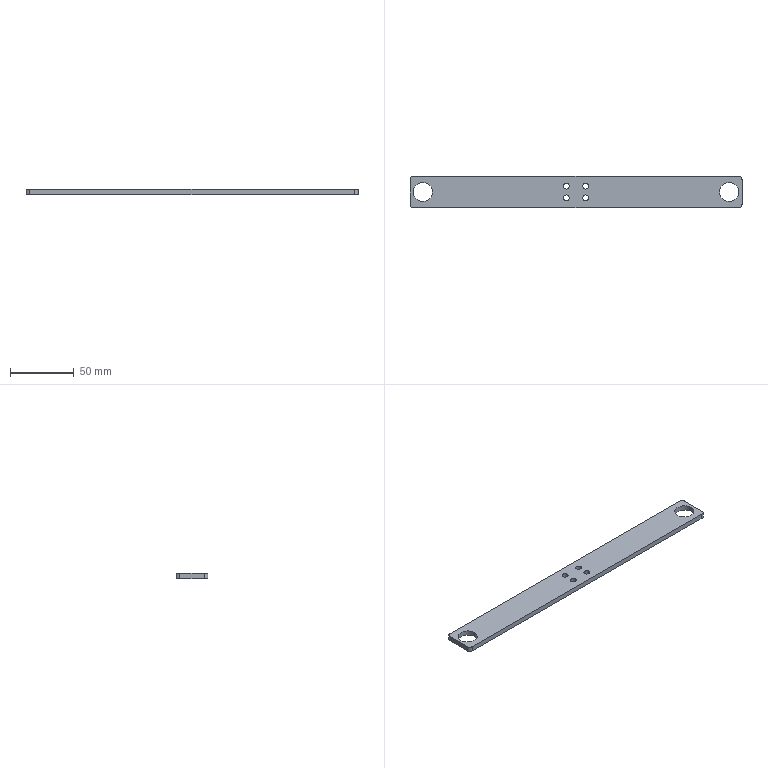Part | SolidWorks | features BaseBody 1 | 1 solid | 22 faces | box 260 x 25 x 4 mm | volume 24301 mm3 | cylinder 16 | plane 6 | commonest cylinder face diameters 4.5 x8 6 x4 15 x4
STEP:
#1=CARTESIAN_POINT('',(-127.5,0.,0.));
#2=VERTEX_POINT('',#1);
#3=CARTESIAN_POINT('',(-127.5,0.,4.));
#4=VERTEX_POINT('',#3);
#5=CARTESIAN_POINT('',(-127.5,0.,4.));
#6=DIRECTION('',(0.,0.,1.));
#7=VECTOR('',#6,1000.);
#8=LINE('',#5,#7);
#9=EDGE_CURVE('',#2,#4,#8,.T.);
#10=ORIENTED_EDGE('',*,*,#9,.F.);
#11=CARTESIAN_POINT('',(-112.5,0.,0.));
#12=VERTEX_POINT('',#11);
#13=CARTESIAN_POINT('',(-120.,0.,0.));
#14=DIRECTION('',(0.,0.,1.));
#15=DIRECTION('',(1.,0.,0.));
#16=AXIS2_PLACEMENT_3D('',#13,#14,#15);
#17=CIRCLE('',#16,7.5);
#18=EDGE_CURVE('',#12,#2,#17,.T.);
#19=ORIENTED_EDGE('',*,*,#18,.F.);
#20=CARTESIAN_POINT('',(-112.5,0.,4.));
#21=VERTEX_POINT('',#20);
#22=CARTESIAN_POINT('',(-112.5,0.,4.));
#23=DIRECTION('',(0.,0.,1.));
#24=VECTOR('',#23,1000.);
#25=LINE('',#22,#24);
#26=EDGE_CURVE('',#12,#21,#25,.T.);
#27=ORIENTED_EDGE('',*,*,#26,.T.);
#28=CARTESIAN_POINT('',(-120.,0.,4.));
#29=DIRECTION('',(0.,0.,1.));
#30=DIRECTION('',(1.,0.,0.));
#31=AXIS2_PLACEMENT_3D('',#28,#29,#30);
#32=CIRCLE('',#31,7.5);
#33=EDGE_CURVE('',#21,#4,#32,.T.);
#34=ORIENTED_EDGE('',*,*,#33,.T.);
#35=EDGE_LOOP('',(#10,#19,#27,#34));
#36=FACE_OUTER_BOUND('',#35,.T.);
#37=CARTESIAN_POINT('',(-120.,0.,4.));
#38=DIRECTION('',(0.,0.,1.));
#39=DIRECTION('',(1.,0.,0.));
#40=AXIS2_PLACEMENT_3D('',#37,#38,#39);
#41=CYLINDRICAL_SURFACE('',#40,7.5);
#42=ADVANCED_FACE('',(#36),#41,.F.);
#43=CARTESIAN_POINT('',(112.5,0.,0.));
#44=VERTEX_POINT('',#43);
#45=CARTESIAN_POINT('',(112.5,0.,4.));
#46=VERTEX_POINT('',#45);
#47=CARTESIAN_POINT('',(112.5,0.,4.));
#48=DIRECTION('',(0.,0.,1.));
#49=VECTOR('',#48,1000.);
#50=LINE('',#47,#49);
#51=EDGE_CURVE('',#44,#46,#50,.T.);
#52=ORIENTED_EDGE('',*,*,#51,.F.);
#53=CARTESIAN_POINT('',(127.5,0.,0.));
#54=VERTEX_POINT('',#53);
#55=CARTESIAN_POINT('',(120.,0.,0.));
#56=DIRECTION('',(0.,0.,1.));
#57=DIRECTION('',(1.,0.,0.));
#58=AXIS2_PLACEMENT_3D('',#55,#56,#57);
#59=CIRCLE('',#58,7.5);
#60=EDGE_CURVE('',#54,#44,#59,.T.);
#61=ORIENTED_EDGE('',*,*,#60,.F.);
#62=CARTESIAN_POINT('',(127.5,0.,4.));
#63=VERTEX_POINT('',#62);
#64=CARTESIAN_POINT('',(127.5,0.,4.));
#65=DIRECTION('',(0.,0.,1.));
#66=VECTOR('',#65,1000.);
#67=LINE('',#64,#66);
#68=EDGE_CURVE('',#54,#63,#67,.T.);
#69=ORIENTED_EDGE('',*,*,#68,.T.);
#70=CARTESIAN_POINT('',(120.,0.,4.));
#71=DIRECTION('',(0.,0.,1.));
#72=DIRECTION('',(1.,0.,0.));
#73=AXIS2_PLACEMENT_3D('',#70,#71,#72);
#74=CIRCLE('',#73,7.5);
#75=EDGE_CURVE('',#63,#46,#74,.T.);
#76=ORIENTED_EDGE('',*,*,#75,.T.);
#77=EDGE_LOOP('',(#52,#61,#69,#76));
#78=FACE_OUTER_BOUND('',#77,.T.);
#79=CARTESIAN_POINT('',(120.,0.,4.));
#80=DIRECTION('',(0.,0.,1.));
#81=DIRECTION('',(1.,0.,0.));
#82=AXIS2_PLACEMENT_3D('',#79,#80,#81);
#83=CYLINDRICAL_SURFACE('',#82,7.5);
#84=ADVANCED_FACE('',(#78),#83,.F.);
#85=CARTESIAN_POINT('',(-9.75,4.5,0.));
#86=VERTEX_POINT('',#85);
#87=CARTESIAN_POINT('',(-9.75,4.5,4.));
#88=VERTEX_POINT('',#87);
#89=CARTESIAN_POINT('',(-9.75,4.5,4.));
#90=DIRECTION('',(0.,0.,1.));
#91=VECTOR('',#90,1000.);
#92=LINE('',#89,#91);
#93=EDGE_CURVE('',#86,#88,#92,.T.);
#94=ORIENTED_EDGE('',*,*,#93,.F.);
#95=CARTESIAN_POINT('',(-5.25,4.5,0.));
#96=VERTEX_POINT('',#95);
#97=CARTESIAN_POINT('',(-7.5,4.5,0.));
#98=DIRECTION('',(0.,0.,1.));
#99=DIRECTION('',(1.,0.,0.));
#100=AXIS2_PLACEMENT_3D('',#97,#98,#99);
#101=CIRCLE('',#100,2.25);
#102=EDGE_CURVE('',#96,#86,#101,.T.);
#103=ORIENTED_EDGE('',*,*,#102,.F.);
#104=CARTESIAN_POINT('',(-5.25,4.5,4.));
#105=VERTEX_POINT('',#104);
#106=CARTESIAN_POINT('',(-5.25,4.5,4.));
#107=DIRECTION('',(0.,0.,1.));
#108=VECTOR('',#107,1000.);
#109=LINE('',#106,#108);
#110=EDGE_CURVE('',#96,#105,#109,.T.);
#111=ORIENTED_EDGE('',*,*,#110,.T.);
#112=CARTESIAN_POINT('',(-7.5,4.5,4.));
#113=DIRECTION('',(0.,0.,1.));
#114=DIRECTION('',(1.,0.,0.));
#115=AXIS2_PLACEMENT_3D('',#112,#113,#114);
#116=CIRCLE('',#115,2.25);
#117=EDGE_CURVE('',#105,#88,#116,.T.);
#118=ORIENTED_EDGE('',*,*,#117,.T.);
#119=EDGE_LOOP('',(#94,#103,#111,#118));
#120=FACE_OUTER_BOUND('',#119,.T.);
#121=CARTESIAN_POINT('',(-7.5,4.5,4.));
#122=DIRECTION('',(0.,0.,1.));
#123=DIRECTION('',(1.,0.,0.));
#124=AXIS2_PLACEMENT_3D('',#121,#122,#123);
#125=CYLINDRICAL_SURFACE('',#124,2.25);
#126=ADVANCED_FACE('',(#120),#125,.F.);
#127=CARTESIAN_POINT('',(-9.75,-4.5,0.));
#128=VERTEX_POINT('',#127);
#129=CARTESIAN_POINT('',(-9.75,-4.5,4.));
#130=VERTEX_POINT('',#129);
#131=CARTESIAN_POINT('',(-9.75,-4.5,4.));
#132=DIRECTION('',(0.,0.,1.));
#133=VECTOR('',#132,1000.);
#134=LINE('',#131,#133);
#135=EDGE_CURVE('',#128,#130,#134,.T.);
#136=ORIENTED_EDGE('',*,*,#135,.F.);
#137=CARTESIAN_POINT('',(-5.25,-4.5,0.));
#138=VERTEX_POINT('',#137);
#139=CARTESIAN_POINT('',(-7.5,-4.5,0.));
#140=DIRECTION('',(0.,0.,1.));
#141=DIRECTION('',(1.,0.,0.));
#142=AXIS2_PLACEMENT_3D('',#139,#140,#141);
#143=CIRCLE('',#142,2.25);
#144=EDGE_CURVE('',#138,#128,#143,.T.);
#145=ORIENTED_EDGE('',*,*,#144,.F.);
#146=CARTESIAN_POINT('',(-5.25,-4.5,4.));
#147=VERTEX_POINT('',#146);
#148=CARTESIAN_POINT('',(-5.25,-4.5,4.));
#149=DIRECTION('',(0.,0.,1.));
#150=VECTOR('',#149,1000.);
#151=LINE('',#148,#150);
#152=EDGE_CURVE('',#138,#147,#151,.T.);
#153=ORIENTED_EDGE('',*,*,#152,.T.);
#154=CARTESIAN_POINT('',(-7.5,-4.5,4.));
#155=DIRECTION('',(0.,0.,1.));
#156=DIRECTION('',(1.,0.,0.));
#157=AXIS2_PLACEMENT_3D('',#154,#155,#156);
#158=CIRCLE('',#157,2.25);
#159=EDGE_CURVE('',#147,#130,#158,.T.);
#160=ORIENTED_EDGE('',*,*,#159,.T.);
#161=EDGE_LOOP('',(#136,#145,#153,#160));
#162=FACE_OUTER_BOUND('',#161,.T.);
#163=CARTESIAN_POINT('',(-7.5,-4.5,4.));
#164=DIRECTION('',(0.,0.,1.));
#165=DIRECTION('',(1.,0.,0.));
#166=AXIS2_PLACEMENT_3D('',#163,#164,#165);
#167=CYLINDRICAL_SURFACE('',#166,2.25);
#168=ADVANCED_FACE('',(#162),#167,.F.);
#169=CARTESIAN_POINT('',(5.25,-4.5,0.));
#170=VERTEX_POINT('',#169);
#171=CARTESIAN_POINT('',(5.25,-4.5,4.));
#172=VERTEX_POINT('',#171);
#173=CARTESIAN_POINT('',(5.25,-4.5,4.));
#174=DIRECTION('',(0.,0.,1.));
#175=VECTOR('',#174,1000.);
#176=LINE('',#173,#175);
#177=EDGE_CURVE('',#170,#172,#176,.T.);
#178=ORIENTED_EDGE('',*,*,#177,.F.);
#179=CARTESIAN_POINT('',(9.75,-4.5,0.));
#180=VERTEX_POINT('',#179);
#181=CARTESIAN_POINT('',(7.5,-4.5,0.));
#182=DIRECTION('',(0.,0.,1.));
#183=DIRECTION('',(1.,0.,0.));
#184=AXIS2_PLACEMENT_3D('',#181,#182,#183);
#185=CIRCLE('',#184,2.25);
#186=EDGE_CURVE('',#180,#170,#185,.T.);
#187=ORIENTED_EDGE('',*,*,#186,.F.);
#188=CARTESIAN_POINT('',(9.75,-4.5,4.));
#189=VERTEX_POINT('',#188);
#190=CARTESIAN_POINT('',(9.75,-4.5,4.));
#191=DIRECTION('',(0.,0.,1.));
#192=VECTOR('',#191,1000.);
#193=LINE('',#190,#192);
#194=EDGE_CURVE('',#180,#189,#193,.T.);
#195=ORIENTED_EDGE('',*,*,#194,.T.);
#196=CARTESIAN_POINT('',(7.5,-4.5,4.));
#197=DIRECTION('',(0.,0.,1.));
#198=DIRECTION('',(1.,0.,0.));
#199=AXIS2_PLACEMENT_3D('',#196,#197,#198);
#200=CIRCLE('',#199,2.25);
#201=EDGE_CURVE('',#189,#172,#200,.T.);
#202=ORIENTED_EDGE('',*,*,#201,.T.);
#203=EDGE_LOOP('',(#178,#187,#195,#202));
#204=FACE_OUTER_BOUND('',#203,.T.);
#205=CARTESIAN_POINT('',(7.5,-4.5,4.));
#206=DIRECTION('',(0.,0.,1.));
#207=DIRECTION('',(1.,0.,0.));
#208=AXIS2_PLACEMENT_3D('',#205,#206,#207);
#209=CYLINDRICAL_SURFACE('',#208,2.25);
#210=ADVANCED_FACE('',(#204),#209,.F.);
#211=CARTESIAN_POINT('',(5.25,4.5,0.));
#212=VERTEX_POINT('',#211);
#213=CARTESIAN_POINT('',(5.25,4.5,4.));
#214=VERTEX_POINT('',#213);
#215=CARTESIAN_POINT('',(5.25,4.5,4.));
#216=DIRECTION('',(0.,0.,1.));
#217=VECTOR('',#216,1000.);
#218=LINE('',#215,#217);
#219=EDGE_CURVE('',#212,#214,#218,.T.);
#220=ORIENTED_EDGE('',*,*,#219,.F.);
#221=CARTESIAN_POINT('',(9.75,4.5,0.));
#222=VERTEX_POINT('',#221);
#223=CARTESIAN_POINT('',(7.5,4.5,0.));
#224=DIRECTION('',(0.,0.,1.));
#225=DIRECTION('',(1.,0.,0.));
#226=AXIS2_PLACEMENT_3D('',#223,#224,#225);
#227=CIRCLE('',#226,2.25);
#228=EDGE_CURVE('',#222,#212,#227,.T.);
#229=ORIENTED_EDGE('',*,*,#228,.F.);
#230=CARTESIAN_POINT('',(9.75,4.5,4.));
#231=VERTEX_POINT('',#230);
#232=CARTESIAN_POINT('',(9.75,4.5,4.));
#233=DIRECTION('',(0.,0.,1.));
#234=VECTOR('',#233,1000.);
#235=LINE('',#232,#234);
#236=EDGE_CURVE('',#222,#231,#235,.T.);
#237=ORIENTED_EDGE('',*,*,#236,.T.);
#238=CARTESIAN_POINT('',(7.5,4.5,4.));
#239=DIRECTION('',(0.,0.,1.));
#240=DIRECTION('',(1.,0.,0.));
#241=AXIS2_PLACEMENT_3D('',#238,#239,#240);
#242=CIRCLE('',#241,2.25);
#243=EDGE_CURVE('',#231,#214,#242,.T.);
#244=ORIENTED_EDGE('',*,*,#243,.T.);
#245=EDGE_LOOP('',(#220,#229,#237,#244));
#246=FACE_OUTER_BOUND('',#245,.T.);
#247=CARTESIAN_POINT('',(7.5,4.5,4.));
#248=DIRECTION('',(0.,0.,1.));
#249=DIRECTION('',(1.,0.,0.));
#250=AXIS2_PLACEMENT_3D('',#247,#248,#249);
#251=CYLINDRICAL_SURFACE('',#250,2.25);
#252=ADVANCED_FACE('',(#246),#251,.F.);
#253=CARTESIAN_POINT('',(-130.,-9.5,4.));
#254=VERTEX_POINT('',#253);
#255=CARTESIAN_POINT('',(-127.,-12.5,4.));
#256=VERTEX_POINT('',#255);
#257=CARTESIAN_POINT('',(-127.,-9.5,4.));
#258=DIRECTION('',(0.,0.,1.));
#259=DIRECTION('',(-1.,0.,0.));
#260=AXIS2_PLACEMENT_3D('',#257,#258,#259);
#261=CIRCLE('',#260,3.);
#262=EDGE_CURVE('',#254,#256,#261,.T.);
#263=ORIENTED_EDGE('',*,*,#262,.F.);
#264=CARTESIAN_POINT('',(-130.,-9.5,0.));
#265=VERTEX_POINT('',#264);
#266=CARTESIAN_POINT('',(-130.,-9.5,4.));
#267=DIRECTION('',(0.,0.,1.));
#268=VECTOR('',#267,1000.);
#269=LINE('',#266,#268);
#270=EDGE_CURVE('',#265,#254,#269,.T.);
#271=ORIENTED_EDGE('',*,*,#270,.F.);
#272=CARTESIAN_POINT('',(-127.,-12.5,0.));
#273=VERTEX_POINT('',#272);
#274=CARTESIAN_POINT('',(-127.,-9.5,0.));
#275=DIRECTION('',(0.,0.,-1.));
#276=DIRECTION('',(-1.,0.,0.));
#277=AXIS2_PLACEMENT_3D('',#274,#275,#276);
#278=CIRCLE('',#277,3.);
#279=EDGE_CURVE('',#273,#265,#278,.T.);
#280=ORIENTED_EDGE('',*,*,#279,.F.);
#281=CARTESIAN_POINT('',(-127.,-12.5,4.));
#282=DIRECTION('',(0.,0.,-1.));
#283=VECTOR('',#282,1000.);
#284=LINE('',#281,#283);
#285=EDGE_CURVE('',#256,#273,#284,.T.);
#286=ORIENTED_EDGE('',*,*,#285,.F.);
#287=EDGE_LOOP('',(#263,#271,#280,#286));
#288=FACE_OUTER_BOUND('',#287,.T.);
#289=CARTESIAN_POINT('',(-127.,-9.5,4.));
#290=DIRECTION('',(0.,0.,-1.));
#291=DIRECTION('',(-1.,0.,0.));
#292=AXIS2_PLACEMENT_3D('',#289,#290,#291);
#293=CYLINDRICAL_SURFACE('',#292,3.);
#294=ADVANCED_FACE('',(#288),#293,.T.);
#295=CARTESIAN_POINT('',(-127.,12.5,4.));
#296=VERTEX_POINT('',#295);
#297=CARTESIAN_POINT('',(-130.,9.5,4.));
#298=VERTEX_POINT('',#297);
#299=CARTESIAN_POINT('',(-127.,9.5,4.));
#300=DIRECTION('',(0.,0.,1.));
#301=DIRECTION('',(-1.,0.,0.));
#302=AXIS2_PLACEMENT_3D('',#299,#300,#301);
#303=CIRCLE('',#302,3.);
#304=EDGE_CURVE('',#296,#298,#303,.T.);
#305=ORIENTED_EDGE('',*,*,#304,.F.);
#306=CARTESIAN_POINT('',(-127.,12.5,0.));
#307=VERTEX_POINT('',#306);
#308=CARTESIAN_POINT('',(-127.,12.5,4.));
#309=DIRECTION('',(0.,0.,1.));
#310=VECTOR('',#309,1000.);
#311=LINE('',#308,#310);
#312=EDGE_CURVE('',#307,#296,#311,.T.);
#313=ORIENTED_EDGE('',*,*,#312,.F.);
#314=CARTESIAN_POINT('',(-130.,9.5,0.));
#315=VERTEX_POINT('',#314);
#316=CARTESIAN_POINT('',(-127.,9.5,0.));
#317=DIRECTION('',(0.,0.,-1.));
#318=DIRECTION('',(-1.,0.,0.));
#319=AXIS2_PLACEMENT_3D('',#316,#317,#318);
#320=CIRCLE('',#319,3.);
#321=EDGE_CURVE('',#315,#307,#320,.T.);
#322=ORIENTED_EDGE('',*,*,#321,.F.);
#323=CARTESIAN_POINT('',(-130.,9.5,4.));
#324=DIRECTION('',(0.,0.,-1.));
#325=VECTOR('',#324,1000.);
#326=LINE('',#323,#325);
#327=EDGE_CURVE('',#298,#315,#326,.T.);
#328=ORIENTED_EDGE('',*,*,#327,.F.);
#329=EDGE_LOOP('',(#305,#313,#322,#328));
#330=FACE_OUTER_BOUND('',#329,.T.);
#331=CARTESIAN_POINT('',(-127.,9.5,4.));
#332=DIRECTION('',(0.,0.,-1.));
#333=DIRECTION('',(-1.,0.,0.));
#334=AXIS2_PLACEMENT_3D('',#331,#332,#333);
#335=CYLINDRICAL_SURFACE('',#334,3.);
#336=ADVANCED_FACE('',(#330),#335,.T.);
#337=CARTESIAN_POINT('',(130.,9.5,4.));
#338=VERTEX_POINT('',#337);
#339=CARTESIAN_POINT('',(127.,12.5,4.));
#340=VERTEX_POINT('',#339);
#341=CARTESIAN_POINT('',(127.,9.5,4.));
#342=DIRECTION('',(0.,0.,1.));
#343=DIRECTION('',(-1.,0.,0.));
#344=AXIS2_PLACEMENT_3D('',#341,#342,#343);
#345=CIRCLE('',#344,3.);
#346=EDGE_CURVE('',#338,#340,#345,.T.);
#347=ORIENTED_EDGE('',*,*,#346,.F.);
#348=CARTESIAN_POINT('',(130.,9.5,0.));
#349=VERTEX_POINT('',#348);
#350=CARTESIAN_POINT('',(130.,9.5,4.));
#351=DIRECTION('',(0.,0.,1.));
#352=VECTOR('',#351,1000.);
#353=LINE('',#350,#352);
#354=EDGE_CURVE('',#349,#338,#353,.T.);
#355=ORIENTED_EDGE('',*,*,#354,.F.);
#356=CARTESIAN_POINT('',(127.,12.5,0.));
#357=VERTEX_POINT('',#356);
#358=CARTESIAN_POINT('',(127.,9.5,0.));
#359=DIRECTION('',(0.,0.,-1.));
#360=DIRECTION('',(-1.,0.,0.));
#361=AXIS2_PLACEMENT_3D('',#358,#359,#360);
#362=CIRCLE('',#361,3.);
#363=EDGE_CURVE('',#357,#349,#362,.T.);
#364=ORIENTED_EDGE('',*,*,#363,.F.);
#365=CARTESIAN_POINT('',(127.,12.5,4.));
#366=DIRECTION('',(0.,0.,-1.));
#367=VECTOR('',#366,1000.);
#368=LINE('',#365,#367);
#369=EDGE_CURVE('',#340,#357,#368,.T.);
#370=ORIENTED_EDGE('',*,*,#369,.F.);
#371=EDGE_LOOP('',(#347,#355,#364,#370));
#372=FACE_OUTER_BOUND('',#371,.T.);
#373=CARTESIAN_POINT('',(127.,9.5,4.));
#374=DIRECTION('',(0.,0.,-1.));
#375=DIRECTION('',(-1.,0.,0.));
#376=AXIS2_PLACEMENT_3D('',#373,#374,#375);
#377=CYLINDRICAL_SURFACE('',#376,3.);
#378=ADVANCED_FACE('',(#372),#377,.T.);
#379=CARTESIAN_POINT('',(127.,-12.5,4.));
#380=VERTEX_POINT('',#379);
#381=CARTESIAN_POINT('',(130.,-9.5,4.));
#382=VERTEX_POINT('',#381);
#383=CARTESIAN_POINT('',(127.,-9.5,4.));
#384=DIRECTION('',(0.,0.,1.));
#385=DIRECTION('',(-1.,0.,0.));
#386=AXIS2_PLACEMENT_3D('',#383,#384,#385);
#387=CIRCLE('',#386,3.);
#388=EDGE_CURVE('',#380,#382,#387,.T.);
#389=ORIENTED_EDGE('',*,*,#388,.F.);
#390=CARTESIAN_POINT('',(127.,-12.5,0.));
#391=VERTEX_POINT('',#390);
#392=CARTESIAN_POINT('',(127.,-12.5,4.));
#393=DIRECTION('',(0.,0.,1.));
#394=VECTOR('',#393,1000.);
#395=LINE('',#392,#394);
#396=EDGE_CURVE('',#391,#380,#395,.T.);
#397=ORIENTED_EDGE('',*,*,#396,.F.);
#398=CARTESIAN_POINT('',(130.,-9.5,0.));
#399=VERTEX_POINT('',#398);
#400=CARTESIAN_POINT('',(127.,-9.5,0.));
#401=DIRECTION('',(0.,0.,-1.));
#402=DIRECTION('',(-1.,0.,0.));
#403=AXIS2_PLACEMENT_3D('',#400,#401,#402);
#404=CIRCLE('',#403,3.);
#405=EDGE_CURVE('',#399,#391,#404,.T.);
#406=ORIENTED_EDGE('',*,*,#405,.F.);
#407=CARTESIAN_POINT('',(130.,-9.5,4.));
#408=DIRECTION('',(0.,0.,-1.));
#409=VECTOR('',#408,1000.);
#410=LINE('',#407,#409);
#411=EDGE_CURVE('',#382,#399,#410,.T.);
#412=ORIENTED_EDGE('',*,*,#411,.F.);
#413=EDGE_LOOP('',(#389,#397,#406,#412));
#414=FACE_OUTER_BOUND('',#413,.T.);
#415=CARTESIAN_POINT('',(127.,-9.5,4.));
#416=DIRECTION('',(0.,0.,-1.));
#417=DIRECTION('',(-1.,0.,0.));
#418=AXIS2_PLACEMENT_3D('',#415,#416,#417);
#419=CYLINDRICAL_SURFACE('',#418,3.);
#420=ADVANCED_FACE('',(#414),#419,.T.);
#421=ORIENTED_EDGE('',*,*,#228,.T.);
#422=CARTESIAN_POINT('',(7.5,4.5,0.));
#423=DIRECTION('',(0.,0.,1.));
#424=DIRECTION('',(1.,0.,0.));
#425=AXIS2_PLACEMENT_3D('',#422,#423,#424);
#426=CIRCLE('',#425,2.25);
#427=EDGE_CURVE('',#212,#222,#426,.T.);
#428=ORIENTED_EDGE('',*,*,#427,.T.);
#429=EDGE_LOOP('',(#421,#428));
#430=FACE_BOUND('',#429,.T.);
#431=ORIENTED_EDGE('',*,*,#186,.T.);
#432=CARTESIAN_POINT('',(7.5,-4.5,0.));
#433=DIRECTION('',(0.,0.,1.));
#434=DIRECTION('',(1.,0.,0.));
#435=AXIS2_PLACEMENT_3D('',#432,#433,#434);
#436=CIRCLE('',#435,2.25);
#437=EDGE_CURVE('',#170,#180,#436,.T.);
#438=ORIENTED_EDGE('',*,*,#437,.T.);
#439=EDGE_LOOP('',(#431,#438));
#440=FACE_BOUND('',#439,.T.);
#441=ORIENTED_EDGE('',*,*,#144,.T.);
#442=CARTESIAN_POINT('',(-7.5,-4.5,0.));
#443=DIRECTION('',(0.,0.,1.));
#444=DIRECTION('',(1.,0.,0.));
#445=AXIS2_PLACEMENT_3D('',#442,#443,#444);
#446=CIRCLE('',#445,2.25);
#447=EDGE_CURVE('',#128,#138,#446,.T.);
#448=ORIENTED_EDGE('',*,*,#447,.T.);
#449=EDGE_LOOP('',(#441,#448));
#450=FACE_BOUND('',#449,.T.);
#451=ORIENTED_EDGE('',*,*,#102,.T.);
#452=CARTESIAN_POINT('',(-7.5,4.5,0.));
#453=DIRECTION('',(0.,0.,1.));
#454=DIRECTION('',(1.,0.,0.));
#455=AXIS2_PLACEMENT_3D('',#452,#453,#454);
#456=CIRCLE('',#455,2.25);
#457=EDGE_CURVE('',#86,#96,#456,.T.);
#458=ORIENTED_EDGE('',*,*,#457,.T.);
#459=EDGE_LOOP('',(#451,#458));
#460=FACE_BOUND('',#459,.T.);
#461=ORIENTED_EDGE('',*,*,#60,.T.);
#462=CARTESIAN_POINT('',(120.,0.,0.));
#463=DIRECTION('',(0.,0.,1.));
#464=DIRECTION('',(1.,0.,0.));
#465=AXIS2_PLACEMENT_3D('',#462,#463,#464);
#466=CIRCLE('',#465,7.5);
#467=EDGE_CURVE('',#44,#54,#466,.T.);
#468=ORIENTED_EDGE('',*,*,#467,.T.);
#469=EDGE_LOOP('',(#461,#468));
#470=FACE_BOUND('',#469,.T.);
#471=ORIENTED_EDGE('',*,*,#18,.T.);
#472=CARTESIAN_POINT('',(-120.,0.,0.));
#473=DIRECTION('',(0.,0.,1.));
#474=DIRECTION('',(1.,0.,0.));
#475=AXIS2_PLACEMENT_3D('',#472,#473,#474);
#476=CIRCLE('',#475,7.5);
#477=EDGE_CURVE('',#2,#12,#476,.T.);
#478=ORIENTED_EDGE('',*,*,#477,.T.);
#479=EDGE_LOOP('',(#471,#478));
#480=FACE_BOUND('',#479,.T.);
#481=CARTESIAN_POINT('',(130.,-12.5,0.));
#482=DIRECTION('',(0.,1.,0.));
#483=VECTOR('',#482,1000.);
#484=LINE('',#481,#483);
#485=EDGE_CURVE('',#399,#349,#484,.T.);
#486=ORIENTED_EDGE('',*,*,#485,.F.);
#487=ORIENTED_EDGE('',*,*,#405,.T.);
#488=CARTESIAN_POINT('',(-130.,-12.5,0.));
#489=DIRECTION('',(1.,0.,0.));
#490=VECTOR('',#489,1000.);
#491=LINE('',#488,#490);
#492=EDGE_CURVE('',#273,#391,#491,.T.);
#493=ORIENTED_EDGE('',*,*,#492,.F.);
#494=ORIENTED_EDGE('',*,*,#279,.T.);
#495=CARTESIAN_POINT('',(-130.,-12.5,0.));
#496=DIRECTION('',(0.,-1.,0.));
#497=VECTOR('',#496,1000.);
#498=LINE('',#495,#497);
#499=EDGE_CURVE('',#315,#265,#498,.T.);
#500=ORIENTED_EDGE('',*,*,#499,.F.);
#501=ORIENTED_EDGE('',*,*,#321,.T.);
#502=CARTESIAN_POINT('',(-130.,12.5,0.));
#503=DIRECTION('',(-1.,0.,0.));
#504=VECTOR('',#503,1000.);
#505=LINE('',#502,#504);
#506=EDGE_CURVE('',#357,#307,#505,.T.);
#507=ORIENTED_EDGE('',*,*,#506,.F.);
#508=ORIENTED_EDGE('',*,*,#363,.T.);
#509=EDGE_LOOP('',(#486,#487,#493,#494,#500,#501,#507,#508));
#510=FACE_OUTER_BOUND('',#509,.T.);
#511=CARTESIAN_POINT('',(0.,0.,0.));
#512=DIRECTION('',(0.,0.,-1.));
#513=DIRECTION('',(0.,-1.,0.));
#514=AXIS2_PLACEMENT_3D('',#511,#512,#513);
#515=PLANE('',#514);
#516=ADVANCED_FACE('',(#430,#440,#450,#460,#470,#480,#510),#515,.T.);
#517=ORIENTED_EDGE('',*,*,#492,.T.);
#518=ORIENTED_EDGE('',*,*,#396,.T.);
#519=CARTESIAN_POINT('',(-130.,-12.5,4.));
#520=DIRECTION('',(1.,0.,0.));
#521=VECTOR('',#520,1000.);
#522=LINE('',#519,#521);
#523=EDGE_CURVE('',#256,#380,#522,.T.);
#524=ORIENTED_EDGE('',*,*,#523,.F.);
#525=ORIENTED_EDGE('',*,*,#285,.T.);
#526=EDGE_LOOP('',(#517,#518,#524,#525));
#527=FACE_OUTER_BOUND('',#526,.T.);
#528=CARTESIAN_POINT('',(-130.,-12.5,4.));
#529=DIRECTION('',(0.,1.,0.));
#530=DIRECTION('',(1.,0.,0.));
#531=AXIS2_PLACEMENT_3D('',#528,#529,#530);
#532=PLANE('',#531);
#533=ADVANCED_FACE('',(#527),#532,.F.);
#534=CARTESIAN_POINT('',(-130.,-12.5,4.));
#535=DIRECTION('',(0.,-1.,0.));
#536=VECTOR('',#535,1000.);
#537=LINE('',#534,#536);
#538=EDGE_CURVE('',#298,#254,#537,.T.);
#539=ORIENTED_EDGE('',*,*,#538,.F.);
#540=ORIENTED_EDGE('',*,*,#327,.T.);
#541=ORIENTED_EDGE('',*,*,#499,.T.);
#542=ORIENTED_EDGE('',*,*,#270,.T.);
#543=EDGE_LOOP('',(#539,#540,#541,#542));
#544=FACE_OUTER_BOUND('',#543,.T.);
#545=CARTESIAN_POINT('',(-130.,-12.5,4.));
#546=DIRECTION('',(1.,0.,0.));
#547=DIRECTION('',(0.,1.,0.));
#548=AXIS2_PLACEMENT_3D('',#545,#546,#547);
#549=PLANE('',#548);
#550=ADVANCED_FACE('',(#544),#549,.F.);
#551=CARTESIAN_POINT('',(-130.,12.5,4.));
#552=DIRECTION('',(-1.,0.,0.));
#553=VECTOR('',#552,1000.);
#554=LINE('',#551,#553);
#555=EDGE_CURVE('',#340,#296,#554,.T.);
#556=ORIENTED_EDGE('',*,*,#555,.F.);
#557=ORIENTED_EDGE('',*,*,#369,.T.);
#558=ORIENTED_EDGE('',*,*,#506,.T.);
#559=ORIENTED_EDGE('',*,*,#312,.T.);
#560=EDGE_LOOP('',(#556,#557,#558,#559));
#561=FACE_OUTER_BOUND('',#560,.T.);
#562=CARTESIAN_POINT('',(-130.,12.5,4.));
#563=DIRECTION('',(0.,-1.,0.));
#564=DIRECTION('',(0.,0.,-1.));
#565=AXIS2_PLACEMENT_3D('',#562,#563,#564);
#566=PLANE('',#565);
#567=ADVANCED_FACE('',(#561),#566,.F.);
#568=CARTESIAN_POINT('',(130.,-12.5,4.));
#569=DIRECTION('',(0.,1.,0.));
#570=VECTOR('',#569,1000.);
#571=LINE('',#568,#570);
#572=EDGE_CURVE('',#382,#338,#571,.T.);
#573=ORIENTED_EDGE('',*,*,#572,.F.);
#574=ORIENTED_EDGE('',*,*,#411,.T.);
#575=ORIENTED_EDGE('',*,*,#485,.T.);
#576=ORIENTED_EDGE('',*,*,#354,.T.);
#577=EDGE_LOOP('',(#573,#574,#575,#576));
#578=FACE_OUTER_BOUND('',#577,.T.);
#579=CARTESIAN_POINT('',(130.,-12.5,4.));
#580=DIRECTION('',(-1.,0.,0.));
#581=DIRECTION('',(0.,0.,1.));
#582=AXIS2_PLACEMENT_3D('',#579,#580,#581);
#583=PLANE('',#582);
#584=ADVANCED_FACE('',(#578),#583,.F.);
#585=ORIENTED_EDGE('',*,*,#159,.F.);
#586=CARTESIAN_POINT('',(-7.5,-4.5,4.));
#587=DIRECTION('',(0.,0.,1.));
#588=DIRECTION('',(1.,0.,0.));
#589=AXIS2_PLACEMENT_3D('',#586,#587,#588);
#590=CIRCLE('',#589,2.25);
#591=EDGE_CURVE('',#130,#147,#590,.T.);
#592=ORIENTED_EDGE('',*,*,#591,.F.);
#593=EDGE_LOOP('',(#585,#592));
#594=FACE_BOUND('',#593,.T.);
#595=ORIENTED_EDGE('',*,*,#243,.F.);
#596=CARTESIAN_POINT('',(7.5,4.5,4.));
#597=DIRECTION('',(0.,0.,1.));
#598=DIRECTION('',(1.,0.,0.));
#599=AXIS2_PLACEMENT_3D('',#596,#597,#598);
#600=CIRCLE('',#599,2.25);
#601=EDGE_CURVE('',#214,#231,#600,.T.);
#602=ORIENTED_EDGE('',*,*,#601,.F.);
#603=EDGE_LOOP('',(#595,#602));
#604=FACE_BOUND('',#603,.T.);
#605=ORIENTED_EDGE('',*,*,#201,.F.);
#606=CARTESIAN_POINT('',(7.5,-4.5,4.));
#607=DIRECTION('',(0.,0.,1.));
#608=DIRECTION('',(1.,0.,0.));
#609=AXIS2_PLACEMENT_3D('',#606,#607,#608);
#610=CIRCLE('',#609,2.25);
#611=EDGE_CURVE('',#172,#189,#610,.T.);
#612=ORIENTED_EDGE('',*,*,#611,.F.);
#613=EDGE_LOOP('',(#605,#612));
#614=FACE_BOUND('',#613,.T.);
#615=ORIENTED_EDGE('',*,*,#117,.F.);
#616=CARTESIAN_POINT('',(-7.5,4.5,4.));
#617=DIRECTION('',(0.,0.,1.));
#618=DIRECTION('',(1.,0.,0.));
#619=AXIS2_PLACEMENT_3D('',#616,#617,#618);
#620=CIRCLE('',#619,2.25);
#621=EDGE_CURVE('',#88,#105,#620,.T.);
#622=ORIENTED_EDGE('',*,*,#621,.F.);
#623=EDGE_LOOP('',(#615,#622));
#624=FACE_BOUND('',#623,.T.);
#625=ORIENTED_EDGE('',*,*,#75,.F.);
#626=CARTESIAN_POINT('',(120.,0.,4.));
#627=DIRECTION('',(0.,0.,1.));
#628=DIRECTION('',(1.,0.,0.));
#629=AXIS2_PLACEMENT_3D('',#626,#627,#628);
#630=CIRCLE('',#629,7.5);
#631=EDGE_CURVE('',#46,#63,#630,.T.);
#632=ORIENTED_EDGE('',*,*,#631,.F.);
#633=EDGE_LOOP('',(#625,#632));
#634=FACE_BOUND('',#633,.T.);
#635=ORIENTED_EDGE('',*,*,#33,.F.);
#636=CARTESIAN_POINT('',(-120.,0.,4.));
#637=DIRECTION('',(0.,0.,1.));
#638=DIRECTION('',(1.,0.,0.));
#639=AXIS2_PLACEMENT_3D('',#636,#637,#638);
#640=CIRCLE('',#639,7.5);
#641=EDGE_CURVE('',#4,#21,#640,.T.);
#642=ORIENTED_EDGE('',*,*,#641,.F.);
#643=EDGE_LOOP('',(#635,#642));
#644=FACE_BOUND('',#643,.T.);
#645=ORIENTED_EDGE('',*,*,#523,.T.);
#646=ORIENTED_EDGE('',*,*,#388,.T.);
#647=ORIENTED_EDGE('',*,*,#572,.T.);
#648=ORIENTED_EDGE('',*,*,#346,.T.);
#649=ORIENTED_EDGE('',*,*,#555,.T.);
#650=ORIENTED_EDGE('',*,*,#304,.T.);
#651=ORIENTED_EDGE('',*,*,#538,.T.);
#652=ORIENTED_EDGE('',*,*,#262,.T.);
#653=EDGE_LOOP('',(#645,#646,#647,#648,#649,#650,#651,#652));
#654=FACE_OUTER_BOUND('',#653,.T.);
#655=CARTESIAN_POINT('',(0.,0.,4.));
#656=DIRECTION('',(0.,0.,-1.));
#657=DIRECTION('',(0.,-1.,0.));
#658=AXIS2_PLACEMENT_3D('',#655,#656,#657);
#659=PLANE('',#658);
#660=ADVANCED_FACE('',(#594,#604,#614,#624,#634,#644,#654),#659,.F.);
#661=ORIENTED_EDGE('',*,*,#427,.F.);
#662=ORIENTED_EDGE('',*,*,#219,.T.);
#663=ORIENTED_EDGE('',*,*,#601,.T.);
#664=ORIENTED_EDGE('',*,*,#236,.F.);
#665=EDGE_LOOP('',(#661,#662,#663,#664));
#666=FACE_OUTER_BOUND('',#665,.T.);
#667=CARTESIAN_POINT('',(7.5,4.5,4.));
#668=DIRECTION('',(0.,0.,1.));
#669=DIRECTION('',(1.,0.,0.));
#670=AXIS2_PLACEMENT_3D('',#667,#668,#669);
#671=CYLINDRICAL_SURFACE('',#670,2.25);
#672=ADVANCED_FACE('',(#666),#671,.F.);
#673=ORIENTED_EDGE('',*,*,#437,.F.);
#674=ORIENTED_EDGE('',*,*,#177,.T.);
#675=ORIENTED_EDGE('',*,*,#611,.T.);
#676=ORIENTED_EDGE('',*,*,#194,.F.);
#677=EDGE_LOOP('',(#673,#674,#675,#676));
#678=FACE_OUTER_BOUND('',#677,.T.);
#679=CARTESIAN_POINT('',(7.5,-4.5,4.));
#680=DIRECTION('',(0.,0.,1.));
#681=DIRECTION('',(1.,0.,0.));
#682=AXIS2_PLACEMENT_3D('',#679,#680,#681);
#683=CYLINDRICAL_SURFACE('',#682,2.25);
#684=ADVANCED_FACE('',(#678),#683,.F.);
#685=ORIENTED_EDGE('',*,*,#447,.F.);
#686=ORIENTED_EDGE('',*,*,#135,.T.);
#687=ORIENTED_EDGE('',*,*,#591,.T.);
#688=ORIENTED_EDGE('',*,*,#152,.F.);
#689=EDGE_LOOP('',(#685,#686,#687,#688));
#690=FACE_OUTER_BOUND('',#689,.T.);
#691=CARTESIAN_POINT('',(-7.5,-4.5,4.));
#692=DIRECTION('',(0.,0.,1.));
#693=DIRECTION('',(1.,0.,0.));
#694=AXIS2_PLACEMENT_3D('',#691,#692,#693);
#695=CYLINDRICAL_SURFACE('',#694,2.25);
#696=ADVANCED_FACE('',(#690),#695,.F.);
#697=ORIENTED_EDGE('',*,*,#457,.F.);
#698=ORIENTED_EDGE('',*,*,#93,.T.);
#699=ORIENTED_EDGE('',*,*,#621,.T.);
#700=ORIENTED_EDGE('',*,*,#110,.F.);
#701=EDGE_LOOP('',(#697,#698,#699,#700));
#702=FACE_OUTER_BOUND('',#701,.T.);
#703=CARTESIAN_POINT('',(-7.5,4.5,4.));
#704=DIRECTION('',(0.,0.,1.));
#705=DIRECTION('',(1.,0.,0.));
#706=AXIS2_PLACEMENT_3D('',#703,#704,#705);
#707=CYLINDRICAL_SURFACE('',#706,2.25);
#708=ADVANCED_FACE('',(#702),#707,.F.);
#709=ORIENTED_EDGE('',*,*,#467,.F.);
#710=ORIENTED_EDGE('',*,*,#51,.T.);
#711=ORIENTED_EDGE('',*,*,#631,.T.);
#712=ORIENTED_EDGE('',*,*,#68,.F.);
#713=EDGE_LOOP('',(#709,#710,#711,#712));
#714=FACE_OUTER_BOUND('',#713,.T.);
#715=CARTESIAN_POINT('',(120.,0.,4.));
#716=DIRECTION('',(0.,0.,1.));
#717=DIRECTION('',(1.,0.,0.));
#718=AXIS2_PLACEMENT_3D('',#715,#716,#717);
#719=CYLINDRICAL_SURFACE('',#718,7.5);
#720=ADVANCED_FACE('',(#714),#719,.F.);
#721=ORIENTED_EDGE('',*,*,#477,.F.);
#722=ORIENTED_EDGE('',*,*,#9,.T.);
#723=ORIENTED_EDGE('',*,*,#641,.T.);
#724=ORIENTED_EDGE('',*,*,#26,.F.);
#725=EDGE_LOOP('',(#721,#722,#723,#724));
#726=FACE_OUTER_BOUND('',#725,.T.);
#727=CARTESIAN_POINT('',(-120.,0.,4.));
#728=DIRECTION('',(0.,0.,1.));
#729=DIRECTION('',(1.,0.,0.));
#730=AXIS2_PLACEMENT_3D('',#727,#728,#729);
#731=CYLINDRICAL_SURFACE('',#730,7.5);
#732=ADVANCED_FACE('',(#726),#731,.F.);
#733=CLOSED_SHELL('',(#42,#84,#126,#168,#210,#252,#294,#336,#378,#420,#516,#533,#550,#567,#584,#660,#672,#684,#696,#708,#720,#732));
#734=MANIFOLD_SOLID_BREP('',#733);
#735=CARTESIAN_POINT('',(0.,0.,0.));
#736=DIRECTION('',(0.,0.,1.));
#737=DIRECTION('',(1.,0.,0.));
#738=AXIS2_PLACEMENT_3D('',#735,#736,#737);
#739=(LENGTH_UNIT()NAMED_UNIT(*)SI_UNIT(.MILLI.,.METRE.));
#740=UNCERTAINTY_MEASURE_WITH_UNIT(LENGTH_MEASURE(0.00001),#739,'','');
#741=(NAMED_UNIT(*)PLANE_ANGLE_UNIT()SI_UNIT($,.RADIAN.));
#742=(NAMED_UNIT(*)SI_UNIT($,.STERADIAN.)SOLID_ANGLE_UNIT());
#743=(GEOMETRIC_REPRESENTATION_CONTEXT(3)GLOBAL_UNCERTAINTY_ASSIGNED_CONTEXT((#740))GLOBAL_UNIT_ASSIGNED_CONTEXT((#739,#741,#742))REPRESENTATION_CONTEXT('',''));
#744=ADVANCED_BREP_SHAPE_REPRESENTATION('',(#734,#738),#743);